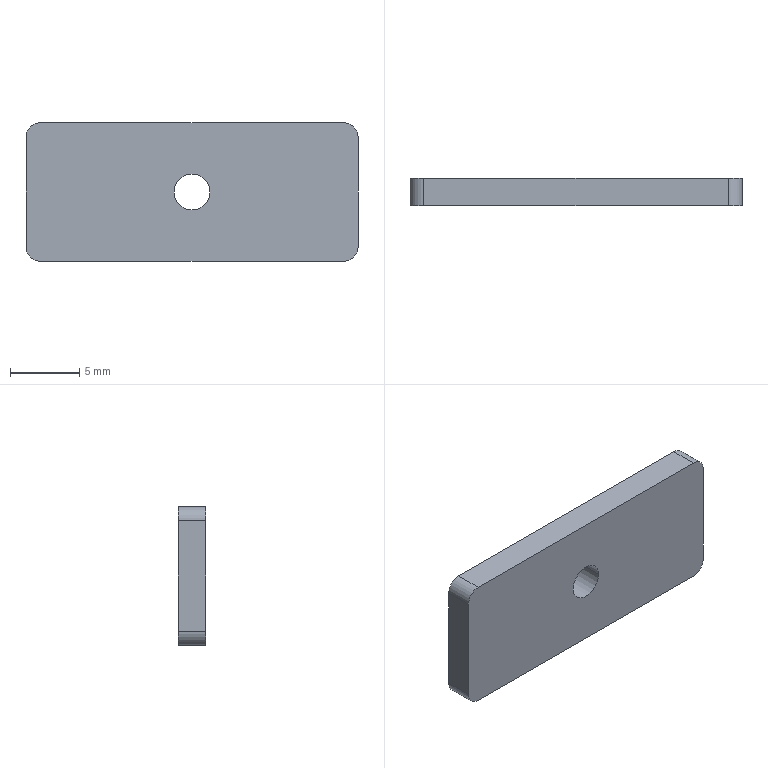Part | STEP file | LRS-150-12_X2_5F00517375-151336 | 1 solid | 12 faces | box 24 x 2 x 10 mm | volume 467.665 mm3 | cylinder 6 | plane 6 | commonest cylinder face diameters 2 x4 2.6 x2
STEP:
#1=CARTESIAN_POINT('',(0.,0.,0.));
#2=DIRECTION('',(0.,0.,1.));
#3=DIRECTION('',(1.,0.,0.));
#4=AXIS2_PLACEMENT_3D('',#1,#2,#3);
#5=CARTESIAN_POINT('',(-242.867,216.425,11.));
#6=VERTEX_POINT('',#5);
#7=CARTESIAN_POINT('',(-245.467,216.425,11.));
#8=VERTEX_POINT('',#7);
#9=CARTESIAN_POINT('',(-244.167,216.425,11.));
#10=DIRECTION('',(0.,-1.,0.));
#11=DIRECTION('',(1.,0.,0.));
#12=AXIS2_PLACEMENT_3D('',#9,#10,#11);
#13=CIRCLE('',#12,1.3);
#14=CARTESIAN_POINT('',(-244.167,214.225,11.));
#15=DIRECTION('',(0.,1.,0.));
#16=DIRECTION('',(1.,0.,0.));
#17=AXIS2_PLACEMENT_3D('',#14,#15,#16);
#18=CYLINDRICAL_SURFACE('',#17,1.3);
#19=CARTESIAN_POINT('',(6.283,2.2));
#20=DIRECTION('',(-1.,0.));
#21=VECTOR('',#20,1.);
#22=LINE('',#19,#21);
#23=(GEOMETRIC_REPRESENTATION_CONTEXT(2)PARAMETRIC_REPRESENTATION_CONTEXT()REPRESENTATION_CONTEXT('',''));
#24=DEFINITIONAL_REPRESENTATION('',(#22),#23);
#25=PCURVE('',#18,#24);
#26=CARTESIAN_POINT('',(-233.336,216.425,14.392));
#27=DIRECTION('',(0.,1.,0.));
#28=DIRECTION('',(1.,0.,0.));
#29=AXIS2_PLACEMENT_3D('',#26,#27,#28);
#30=PLANE('',#29);
#31=CARTESIAN_POINT('',(-9.53,3.392));
#32=CARTESIAN_POINT('',(-9.53,1.14));
#33=CARTESIAN_POINT('',(-11.48,2.266));
#34=CARTESIAN_POINT('',(-13.43,3.392));
#35=CARTESIAN_POINT('',(-11.48,4.517));
#36=CARTESIAN_POINT('',(-9.53,5.643));
#37=CARTESIAN_POINT('',(-9.53,3.392));
#38=(BOUNDED_CURVE()B_SPLINE_CURVE(2,(#31,#32,#33,#34,#35,#36,#37),.UNSPECIFIED.,.T.,.F.)B_SPLINE_CURVE_WITH_KNOTS((1,2,2,2,2,1),(-2.094,0.,2.094,4.189,6.283,8.378),.UNSPECIFIED.)CURVE()GEOMETRIC_REPRESENTATION_ITEM()RATIONAL_B_SPLINE_CURVE((1.,0.5,1.,0.5,1.,0.5,1.))REPRESENTATION_ITEM(''));
#39=(GEOMETRIC_REPRESENTATION_CONTEXT(2)PARAMETRIC_REPRESENTATION_CONTEXT()REPRESENTATION_CONTEXT('',''));
#40=DEFINITIONAL_REPRESENTATION('',(#38),#39);
#41=PCURVE('',#30,#40);
#42=SURFACE_CURVE('',#13,(#25,#41),.PCURVE_S1.);
#43=EDGE_CURVE('',#6,#8,#42,.T.);
#44=ORIENTED_EDGE('',*,*,#43,.T.);
#45=CARTESIAN_POINT('',(-245.467,214.425,11.));
#46=VERTEX_POINT('',#45);
#47=CARTESIAN_POINT('',(-245.467,216.425,11.));
#48=DIRECTION('',(0.,-1.,0.));
#49=VECTOR('',#48,1.);
#50=LINE('',#47,#49);
#51=CARTESIAN_POINT('',(3.142,2.2));
#52=DIRECTION('',(0.,-1.));
#53=VECTOR('',#52,1.);
#54=LINE('',#51,#53);
#55=(GEOMETRIC_REPRESENTATION_CONTEXT(2)PARAMETRIC_REPRESENTATION_CONTEXT()REPRESENTATION_CONTEXT('',''));
#56=DEFINITIONAL_REPRESENTATION('',(#54),#55);
#57=PCURVE('',#18,#56);
#58=CARTESIAN_POINT('',(-244.167,214.225,11.));
#59=DIRECTION('',(0.,1.,0.));
#60=DIRECTION('',(1.,0.,0.));
#61=AXIS2_PLACEMENT_3D('',#58,#59,#60);
#62=CYLINDRICAL_SURFACE('',#61,1.3);
#63=CARTESIAN_POINT('',(3.142,2.2));
#64=DIRECTION('',(0.,-1.));
#65=VECTOR('',#64,1.);
#66=LINE('',#63,#65);
#67=(GEOMETRIC_REPRESENTATION_CONTEXT(2)PARAMETRIC_REPRESENTATION_CONTEXT()REPRESENTATION_CONTEXT('',''));
#68=DEFINITIONAL_REPRESENTATION('',(#66),#67);
#69=PCURVE('',#62,#68);
#70=SURFACE_CURVE('',#50,(#57,#69),.PCURVE_S1.);
#71=EDGE_CURVE('',#8,#46,#70,.T.);
#72=ORIENTED_EDGE('',*,*,#71,.T.);
#73=CARTESIAN_POINT('',(-242.867,214.425,11.));
#74=VERTEX_POINT('',#73);
#75=CARTESIAN_POINT('',(-244.167,214.425,11.));
#76=DIRECTION('',(0.,1.,0.));
#77=DIRECTION('',(-1.,0.,0.));
#78=AXIS2_PLACEMENT_3D('',#75,#76,#77);
#79=CIRCLE('',#78,1.3);
#80=CARTESIAN_POINT('',(3.142,0.2));
#81=DIRECTION('',(1.,0.));
#82=VECTOR('',#81,1.);
#83=LINE('',#80,#82);
#84=(GEOMETRIC_REPRESENTATION_CONTEXT(2)PARAMETRIC_REPRESENTATION_CONTEXT()REPRESENTATION_CONTEXT('',''));
#85=DEFINITIONAL_REPRESENTATION('',(#83),#84);
#86=PCURVE('',#18,#85);
#87=CARTESIAN_POINT('',(-233.336,214.425,14.392));
#88=DIRECTION('',(0.,1.,0.));
#89=DIRECTION('',(1.,0.,0.));
#90=AXIS2_PLACEMENT_3D('',#87,#88,#89);
#91=PLANE('',#90);
#92=CARTESIAN_POINT('',(-10.83,3.392));
#93=DIRECTION('',(-1.,0.));
#94=AXIS2_PLACEMENT_2D('',#92,#93);
#95=CIRCLE('',#94,1.3);
#96=(GEOMETRIC_REPRESENTATION_CONTEXT(2)PARAMETRIC_REPRESENTATION_CONTEXT()REPRESENTATION_CONTEXT('',''));
#97=DEFINITIONAL_REPRESENTATION('',(#95),#96);
#98=PCURVE('',#91,#97);
#99=SURFACE_CURVE('',#79,(#86,#98),.PCURVE_S1.);
#100=EDGE_CURVE('',#46,#74,#99,.T.);
#101=ORIENTED_EDGE('',*,*,#100,.T.);
#102=CARTESIAN_POINT('',(-242.867,216.425,11.));
#103=DIRECTION('',(0.,-1.,0.));
#104=VECTOR('',#103,1.);
#105=LINE('',#102,#104);
#106=CARTESIAN_POINT('',(6.283,2.2));
#107=DIRECTION('',(0.,-1.));
#108=VECTOR('',#107,1.);
#109=LINE('',#106,#108);
#110=(GEOMETRIC_REPRESENTATION_CONTEXT(2)PARAMETRIC_REPRESENTATION_CONTEXT()REPRESENTATION_CONTEXT('',''));
#111=DEFINITIONAL_REPRESENTATION('',(#109),#110);
#112=PCURVE('',#18,#111);
#113=CARTESIAN_POINT('',(0.,2.2));
#114=DIRECTION('',(0.,-1.));
#115=VECTOR('',#114,1.);
#116=LINE('',#113,#115);
#117=(GEOMETRIC_REPRESENTATION_CONTEXT(2)PARAMETRIC_REPRESENTATION_CONTEXT()REPRESENTATION_CONTEXT('',''));
#118=DEFINITIONAL_REPRESENTATION('',(#116),#117);
#119=PCURVE('',#62,#118);
#120=SURFACE_CURVE('',#105,(#112,#119),.PCURVE_S1.);
#121=EDGE_CURVE('',#6,#74,#120,.T.);
#122=ORIENTED_EDGE('',*,*,#121,.F.);
#123=EDGE_LOOP('',(#44,#72,#101,#122));
#124=FACE_BOUND('',#123,.F.);
#125=ADVANCED_FACE('',(#124),#18,.F.);
#126=CARTESIAN_POINT('',(-256.167,216.425,15.));
#127=VERTEX_POINT('',#126);
#128=CARTESIAN_POINT('',(-255.167,216.425,16.));
#129=VERTEX_POINT('',#128);
#130=CARTESIAN_POINT('',(-255.167,216.425,15.));
#131=DIRECTION('',(0.,1.,0.));
#132=DIRECTION('',(-1.,0.,0.));
#133=AXIS2_PLACEMENT_3D('',#130,#131,#132);
#134=CIRCLE('',#133,1.);
#135=CARTESIAN_POINT('',(-21.83,-0.6085));
#136=DIRECTION('',(-1.,0.));
#137=AXIS2_PLACEMENT_2D('',#135,#136);
#138=CIRCLE('',#137,1.);
#139=(GEOMETRIC_REPRESENTATION_CONTEXT(2)PARAMETRIC_REPRESENTATION_CONTEXT()REPRESENTATION_CONTEXT('',''));
#140=DEFINITIONAL_REPRESENTATION('',(#138),#139);
#141=PCURVE('',#30,#140);
#142=CARTESIAN_POINT('',(-255.167,214.425,15.));
#143=DIRECTION('',(0.,1.,0.));
#144=DIRECTION('',(1.,0.,0.));
#145=AXIS2_PLACEMENT_3D('',#142,#143,#144);
#146=CYLINDRICAL_SURFACE('',#145,1.);
#147=CARTESIAN_POINT('',(3.142,2.));
#148=DIRECTION('',(1.,0.));
#149=VECTOR('',#148,1.);
#150=LINE('',#147,#149);
#151=(GEOMETRIC_REPRESENTATION_CONTEXT(2)PARAMETRIC_REPRESENTATION_CONTEXT()REPRESENTATION_CONTEXT('',''));
#152=DEFINITIONAL_REPRESENTATION('',(#150),#151);
#153=PCURVE('',#146,#152);
#154=SURFACE_CURVE('',#134,(#141,#153),.PCURVE_S1.);
#155=EDGE_CURVE('',#127,#129,#154,.T.);
#156=ORIENTED_EDGE('',*,*,#155,.F.);
#157=CARTESIAN_POINT('',(-256.167,216.425,7.));
#158=VERTEX_POINT('',#157);
#159=CARTESIAN_POINT('',(-256.167,216.425,7.));
#160=DIRECTION('',(0.,0.,1.));
#161=VECTOR('',#160,1.);
#162=LINE('',#159,#161);
#163=CARTESIAN_POINT('',(-22.83,7.392));
#164=DIRECTION('',(0.,-1.));
#165=VECTOR('',#164,1.);
#166=LINE('',#163,#165);
#167=(GEOMETRIC_REPRESENTATION_CONTEXT(2)PARAMETRIC_REPRESENTATION_CONTEXT()REPRESENTATION_CONTEXT('',''));
#168=DEFINITIONAL_REPRESENTATION('',(#166),#167);
#169=PCURVE('',#30,#168);
#170=CARTESIAN_POINT('',(-256.167,214.425,16.));
#171=DIRECTION('',(-1.,0.,0.));
#172=DIRECTION('',(0.,0.,1.));
#173=AXIS2_PLACEMENT_3D('',#170,#171,#172);
#174=PLANE('',#173);
#175=CARTESIAN_POINT('',(-9.,2.));
#176=DIRECTION('',(1.,0.));
#177=VECTOR('',#176,1.);
#178=LINE('',#175,#177);
#179=(GEOMETRIC_REPRESENTATION_CONTEXT(2)PARAMETRIC_REPRESENTATION_CONTEXT()REPRESENTATION_CONTEXT('',''));
#180=DEFINITIONAL_REPRESENTATION('',(#178),#179);
#181=PCURVE('',#174,#180);
#182=SURFACE_CURVE('',#162,(#169,#181),.PCURVE_S1.);
#183=EDGE_CURVE('',#158,#127,#182,.T.);
#184=ORIENTED_EDGE('',*,*,#183,.F.);
#185=CARTESIAN_POINT('',(-255.167,216.425,6.));
#186=VERTEX_POINT('',#185);
#187=CARTESIAN_POINT('',(-255.167,216.425,7.));
#188=DIRECTION('',(0.,1.,0.));
#189=DIRECTION('',(0.,0.,-1.));
#190=AXIS2_PLACEMENT_3D('',#187,#188,#189);
#191=CIRCLE('',#190,1.);
#192=CARTESIAN_POINT('',(-21.83,7.392));
#193=DIRECTION('',(0.,1.));
#194=AXIS2_PLACEMENT_2D('',#192,#193);
#195=CIRCLE('',#194,1.);
#196=(GEOMETRIC_REPRESENTATION_CONTEXT(2)PARAMETRIC_REPRESENTATION_CONTEXT()REPRESENTATION_CONTEXT('',''));
#197=DEFINITIONAL_REPRESENTATION('',(#195),#196);
#198=PCURVE('',#30,#197);
#199=CARTESIAN_POINT('',(-255.167,214.425,7.));
#200=DIRECTION('',(0.,1.,0.));
#201=DIRECTION('',(1.,0.,0.));
#202=AXIS2_PLACEMENT_3D('',#199,#200,#201);
#203=CYLINDRICAL_SURFACE('',#202,1.);
#204=CARTESIAN_POINT('',(1.571,2.));
#205=DIRECTION('',(1.,0.));
#206=VECTOR('',#205,1.);
#207=LINE('',#204,#206);
#208=(GEOMETRIC_REPRESENTATION_CONTEXT(2)PARAMETRIC_REPRESENTATION_CONTEXT()REPRESENTATION_CONTEXT('',''));
#209=DEFINITIONAL_REPRESENTATION('',(#207),#208);
#210=PCURVE('',#203,#209);
#211=SURFACE_CURVE('',#191,(#198,#210),.PCURVE_S1.);
#212=EDGE_CURVE('',#186,#158,#211,.T.);
#213=ORIENTED_EDGE('',*,*,#212,.F.);
#214=CARTESIAN_POINT('',(-233.167,216.425,6.));
#215=VERTEX_POINT('',#214);
#216=CARTESIAN_POINT('',(-255.167,216.425,6.));
#217=DIRECTION('',(1.,0.,0.));
#218=VECTOR('',#217,1.);
#219=LINE('',#216,#218);
#220=CARTESIAN_POINT('',(-21.83,8.392));
#221=DIRECTION('',(1.,0.));
#222=VECTOR('',#221,1.);
#223=LINE('',#220,#222);
#224=(GEOMETRIC_REPRESENTATION_CONTEXT(2)PARAMETRIC_REPRESENTATION_CONTEXT()REPRESENTATION_CONTEXT('',''));
#225=DEFINITIONAL_REPRESENTATION('',(#223),#224);
#226=PCURVE('',#30,#225);
#227=CARTESIAN_POINT('',(-261.667,214.425,6.));
#228=DIRECTION('',(0.,0.,-1.));
#229=DIRECTION('',(-1.,0.,0.));
#230=AXIS2_PLACEMENT_3D('',#227,#228,#229);
#231=PLANE('',#230);
#232=CARTESIAN_POINT('',(-6.5,2.));
#233=DIRECTION('',(-1.,0.));
#234=VECTOR('',#233,1.);
#235=LINE('',#232,#234);
#236=(GEOMETRIC_REPRESENTATION_CONTEXT(2)PARAMETRIC_REPRESENTATION_CONTEXT()REPRESENTATION_CONTEXT('',''));
#237=DEFINITIONAL_REPRESENTATION('',(#235),#236);
#238=PCURVE('',#231,#237);
#239=SURFACE_CURVE('',#219,(#226,#238),.PCURVE_S1.);
#240=EDGE_CURVE('',#186,#215,#239,.T.);
#241=ORIENTED_EDGE('',*,*,#240,.T.);
#242=CARTESIAN_POINT('',(-232.167,216.425,7.));
#243=VERTEX_POINT('',#242);
#244=CARTESIAN_POINT('',(-233.167,216.425,7.));
#245=DIRECTION('',(0.,1.,0.));
#246=DIRECTION('',(1.,0.,0.));
#247=AXIS2_PLACEMENT_3D('',#244,#245,#246);
#248=CIRCLE('',#247,1.);
#249=CARTESIAN_POINT('',(0.1696,7.392));
#250=DIRECTION('',(1.,0.));
#251=AXIS2_PLACEMENT_2D('',#249,#250);
#252=CIRCLE('',#251,1.);
#253=(GEOMETRIC_REPRESENTATION_CONTEXT(2)PARAMETRIC_REPRESENTATION_CONTEXT()REPRESENTATION_CONTEXT('',''));
#254=DEFINITIONAL_REPRESENTATION('',(#252),#253);
#255=PCURVE('',#30,#254);
#256=CARTESIAN_POINT('',(-233.167,214.425,7.));
#257=DIRECTION('',(0.,1.,0.));
#258=DIRECTION('',(1.,0.,0.));
#259=AXIS2_PLACEMENT_3D('',#256,#257,#258);
#260=CYLINDRICAL_SURFACE('',#259,1.);
#261=CARTESIAN_POINT('',(0.,2.));
#262=DIRECTION('',(1.,0.));
#263=VECTOR('',#262,1.);
#264=LINE('',#261,#263);
#265=(GEOMETRIC_REPRESENTATION_CONTEXT(2)PARAMETRIC_REPRESENTATION_CONTEXT()REPRESENTATION_CONTEXT('',''));
#266=DEFINITIONAL_REPRESENTATION('',(#264),#265);
#267=PCURVE('',#260,#266);
#268=SURFACE_CURVE('',#248,(#255,#267),.PCURVE_S1.);
#269=EDGE_CURVE('',#243,#215,#268,.T.);
#270=ORIENTED_EDGE('',*,*,#269,.F.);
#271=CARTESIAN_POINT('',(-232.167,216.425,15.));
#272=VERTEX_POINT('',#271);
#273=CARTESIAN_POINT('',(-232.167,216.425,15.));
#274=DIRECTION('',(0.,0.,-1.));
#275=VECTOR('',#274,1.);
#276=LINE('',#273,#275);
#277=CARTESIAN_POINT('',(1.17,-0.6085));
#278=DIRECTION('',(0.,1.));
#279=VECTOR('',#278,1.);
#280=LINE('',#277,#279);
#281=(GEOMETRIC_REPRESENTATION_CONTEXT(2)PARAMETRIC_REPRESENTATION_CONTEXT()REPRESENTATION_CONTEXT('',''));
#282=DEFINITIONAL_REPRESENTATION('',(#280),#281);
#283=PCURVE('',#30,#282);
#284=CARTESIAN_POINT('',(-232.167,214.425,6.));
#285=DIRECTION('',(1.,0.,0.));
#286=DIRECTION('',(0.,0.,-1.));
#287=AXIS2_PLACEMENT_3D('',#284,#285,#286);
#288=PLANE('',#287);
#289=CARTESIAN_POINT('',(-9.,2.));
#290=DIRECTION('',(1.,0.));
#291=VECTOR('',#290,1.);
#292=LINE('',#289,#291);
#293=(GEOMETRIC_REPRESENTATION_CONTEXT(2)PARAMETRIC_REPRESENTATION_CONTEXT()REPRESENTATION_CONTEXT('',''));
#294=DEFINITIONAL_REPRESENTATION('',(#292),#293);
#295=PCURVE('',#288,#294);
#296=SURFACE_CURVE('',#276,(#283,#295),.PCURVE_S1.);
#297=EDGE_CURVE('',#272,#243,#296,.T.);
#298=ORIENTED_EDGE('',*,*,#297,.F.);
#299=CARTESIAN_POINT('',(-233.167,216.425,16.));
#300=VERTEX_POINT('',#299);
#301=CARTESIAN_POINT('',(-233.167,216.425,15.));
#302=DIRECTION('',(0.,1.,0.));
#303=DIRECTION('',(0.,0.,1.));
#304=AXIS2_PLACEMENT_3D('',#301,#302,#303);
#305=CIRCLE('',#304,1.);
#306=CARTESIAN_POINT('',(0.1696,-0.6085));
#307=DIRECTION('',(0.,-1.));
#308=AXIS2_PLACEMENT_2D('',#306,#307);
#309=CIRCLE('',#308,1.);
#310=(GEOMETRIC_REPRESENTATION_CONTEXT(2)PARAMETRIC_REPRESENTATION_CONTEXT()REPRESENTATION_CONTEXT('',''));
#311=DEFINITIONAL_REPRESENTATION('',(#309),#310);
#312=PCURVE('',#30,#311);
#313=CARTESIAN_POINT('',(-233.167,214.425,15.));
#314=DIRECTION('',(0.,1.,0.));
#315=DIRECTION('',(1.,0.,0.));
#316=AXIS2_PLACEMENT_3D('',#313,#314,#315);
#317=CYLINDRICAL_SURFACE('',#316,1.);
#318=CARTESIAN_POINT('',(4.712,2.));
#319=DIRECTION('',(1.,0.));
#320=VECTOR('',#319,1.);
#321=LINE('',#318,#320);
#322=(GEOMETRIC_REPRESENTATION_CONTEXT(2)PARAMETRIC_REPRESENTATION_CONTEXT()REPRESENTATION_CONTEXT('',''));
#323=DEFINITIONAL_REPRESENTATION('',(#321),#322);
#324=PCURVE('',#317,#323);
#325=SURFACE_CURVE('',#305,(#312,#324),.PCURVE_S1.);
#326=EDGE_CURVE('',#300,#272,#325,.T.);
#327=ORIENTED_EDGE('',*,*,#326,.F.);
#328=CARTESIAN_POINT('',(-233.167,216.425,16.));
#329=DIRECTION('',(-1.,0.,0.));
#330=VECTOR('',#329,1.);
#331=LINE('',#328,#330);
#332=CARTESIAN_POINT('',(0.1696,-1.608));
#333=DIRECTION('',(-1.,0.));
#334=VECTOR('',#333,1.);
#335=LINE('',#332,#334);
#336=(GEOMETRIC_REPRESENTATION_CONTEXT(2)PARAMETRIC_REPRESENTATION_CONTEXT()REPRESENTATION_CONTEXT('',''));
#337=DEFINITIONAL_REPRESENTATION('',(#335),#336);
#338=PCURVE('',#30,#337);
#339=CARTESIAN_POINT('',(-226.667,214.425,16.));
#340=DIRECTION('',(0.,0.,1.));
#341=DIRECTION('',(1.,0.,0.));
#342=AXIS2_PLACEMENT_3D('',#339,#340,#341);
#343=PLANE('',#342);
#344=CARTESIAN_POINT('',(-6.5,2.));
#345=DIRECTION('',(-1.,0.));
#346=VECTOR('',#345,1.);
#347=LINE('',#344,#346);
#348=(GEOMETRIC_REPRESENTATION_CONTEXT(2)PARAMETRIC_REPRESENTATION_CONTEXT()REPRESENTATION_CONTEXT('',''));
#349=DEFINITIONAL_REPRESENTATION('',(#347),#348);
#350=PCURVE('',#343,#349);
#351=SURFACE_CURVE('',#331,(#338,#350),.PCURVE_S1.);
#352=EDGE_CURVE('',#300,#129,#351,.T.);
#353=ORIENTED_EDGE('',*,*,#352,.T.);
#354=EDGE_LOOP('',(#156,#184,#213,#241,#270,#298,#327,#353));
#355=FACE_BOUND('',#354,.F.);
#356=ORIENTED_EDGE('',*,*,#43,.F.);
#357=CARTESIAN_POINT('',(-244.167,216.425,11.));
#358=DIRECTION('',(0.,-1.,0.));
#359=DIRECTION('',(-1.,0.,0.));
#360=AXIS2_PLACEMENT_3D('',#357,#358,#359);
#361=CIRCLE('',#360,1.3);
#362=CARTESIAN_POINT('',(-12.13,3.392));
#363=CARTESIAN_POINT('',(-12.13,5.643));
#364=CARTESIAN_POINT('',(-10.18,4.517));
#365=CARTESIAN_POINT('',(-8.23,3.392));
#366=CARTESIAN_POINT('',(-10.18,2.266));
#367=CARTESIAN_POINT('',(-12.13,1.14));
#368=CARTESIAN_POINT('',(-12.13,3.392));
#369=(BOUNDED_CURVE()B_SPLINE_CURVE(2,(#362,#363,#364,#365,#366,#367,#368),.UNSPECIFIED.,.T.,.F.)B_SPLINE_CURVE_WITH_KNOTS((1,2,2,2,2,1),(-2.094,0.,2.094,4.189,6.283,8.378),.UNSPECIFIED.)CURVE()GEOMETRIC_REPRESENTATION_ITEM()RATIONAL_B_SPLINE_CURVE((1.,0.5,1.,0.5,1.,0.5,1.))REPRESENTATION_ITEM(''));
#370=(GEOMETRIC_REPRESENTATION_CONTEXT(2)PARAMETRIC_REPRESENTATION_CONTEXT()REPRESENTATION_CONTEXT('',''));
#371=DEFINITIONAL_REPRESENTATION('',(#369),#370);
#372=PCURVE('',#30,#371);
#373=CARTESIAN_POINT('',(3.142,2.2));
#374=DIRECTION('',(-1.,0.));
#375=VECTOR('',#374,1.);
#376=LINE('',#373,#375);
#377=(GEOMETRIC_REPRESENTATION_CONTEXT(2)PARAMETRIC_REPRESENTATION_CONTEXT()REPRESENTATION_CONTEXT('',''));
#378=DEFINITIONAL_REPRESENTATION('',(#376),#377);
#379=PCURVE('',#62,#378);
#380=SURFACE_CURVE('',#361,(#372,#379),.PCURVE_S1.);
#381=EDGE_CURVE('',#8,#6,#380,.T.);
#382=ORIENTED_EDGE('',*,*,#381,.F.);
#383=EDGE_LOOP('',(#356,#382));
#384=FACE_BOUND('',#383,.F.);
#385=ADVANCED_FACE('',(#355,#384),#30,.T.);
#386=ORIENTED_EDGE('',*,*,#121,.T.);
#387=CARTESIAN_POINT('',(-244.167,214.425,11.));
#388=DIRECTION('',(0.,1.,0.));
#389=DIRECTION('',(1.,0.,0.));
#390=AXIS2_PLACEMENT_3D('',#387,#388,#389);
#391=CIRCLE('',#390,1.3);
#392=CARTESIAN_POINT('',(0.,0.2));
#393=DIRECTION('',(1.,0.));
#394=VECTOR('',#393,1.);
#395=LINE('',#392,#394);
#396=(GEOMETRIC_REPRESENTATION_CONTEXT(2)PARAMETRIC_REPRESENTATION_CONTEXT()REPRESENTATION_CONTEXT('',''));
#397=DEFINITIONAL_REPRESENTATION('',(#395),#396);
#398=PCURVE('',#62,#397);
#399=CARTESIAN_POINT('',(-10.83,3.392));
#400=DIRECTION('',(1.,0.));
#401=AXIS2_PLACEMENT_2D('',#399,#400);
#402=CIRCLE('',#401,1.3);
#403=(GEOMETRIC_REPRESENTATION_CONTEXT(2)PARAMETRIC_REPRESENTATION_CONTEXT()REPRESENTATION_CONTEXT('',''));
#404=DEFINITIONAL_REPRESENTATION('',(#402),#403);
#405=PCURVE('',#91,#404);
#406=SURFACE_CURVE('',#391,(#398,#405),.PCURVE_S1.);
#407=EDGE_CURVE('',#74,#46,#406,.T.);
#408=ORIENTED_EDGE('',*,*,#407,.T.);
#409=ORIENTED_EDGE('',*,*,#71,.F.);
#410=ORIENTED_EDGE('',*,*,#381,.T.);
#411=EDGE_LOOP('',(#386,#408,#409,#410));
#412=FACE_BOUND('',#411,.F.);
#413=ADVANCED_FACE('',(#412),#62,.F.);
#414=CARTESIAN_POINT('',(-233.167,214.425,6.));
#415=VERTEX_POINT('',#414);
#416=CARTESIAN_POINT('',(-232.167,214.425,7.));
#417=VERTEX_POINT('',#416);
#418=CARTESIAN_POINT('',(-233.167,214.425,7.));
#419=DIRECTION('',(0.,-1.,0.));
#420=DIRECTION('',(0.,0.,-1.));
#421=AXIS2_PLACEMENT_3D('',#418,#419,#420);
#422=CIRCLE('',#421,1.);
#423=CARTESIAN_POINT('',(0.1696,8.392));
#424=CARTESIAN_POINT('',(1.902,8.392));
#425=CARTESIAN_POINT('',(1.036,6.892));
#426=CARTESIAN_POINT('',(0.1696,5.392));
#427=CARTESIAN_POINT('',(-0.6964,6.892));
#428=CARTESIAN_POINT('',(-1.562,8.392));
#429=CARTESIAN_POINT('',(0.1696,8.392));
#430=(BOUNDED_CURVE()B_SPLINE_CURVE(2,(#423,#424,#425,#426,#427,#428,#429),.UNSPECIFIED.,.T.,.F.)B_SPLINE_CURVE_WITH_KNOTS((1,2,2,2,2,1),(-2.094,0.,2.094,4.189,6.283,8.378),.UNSPECIFIED.)CURVE()GEOMETRIC_REPRESENTATION_ITEM()RATIONAL_B_SPLINE_CURVE((1.,0.5,1.,0.5,1.,0.5,1.))REPRESENTATION_ITEM(''));
#431=(GEOMETRIC_REPRESENTATION_CONTEXT(2)PARAMETRIC_REPRESENTATION_CONTEXT()REPRESENTATION_CONTEXT('',''));
#432=DEFINITIONAL_REPRESENTATION('',(#430),#431);
#433=PCURVE('',#91,#432);
#434=CARTESIAN_POINT('',(1.571,0.));
#435=DIRECTION('',(-1.,0.));
#436=VECTOR('',#435,1.);
#437=LINE('',#434,#436);
#438=(GEOMETRIC_REPRESENTATION_CONTEXT(2)PARAMETRIC_REPRESENTATION_CONTEXT()REPRESENTATION_CONTEXT('',''));
#439=DEFINITIONAL_REPRESENTATION('',(#437),#438);
#440=PCURVE('',#260,#439);
#441=SURFACE_CURVE('',#422,(#433,#440),.PCURVE_S1.);
#442=EDGE_CURVE('',#415,#417,#441,.T.);
#443=ORIENTED_EDGE('',*,*,#442,.F.);
#444=CARTESIAN_POINT('',(-255.167,214.425,6.));
#445=VERTEX_POINT('',#444);
#446=CARTESIAN_POINT('',(-255.167,214.425,6.));
#447=DIRECTION('',(1.,0.,0.));
#448=VECTOR('',#447,1.);
#449=LINE('',#446,#448);
#450=CARTESIAN_POINT('',(-21.83,8.392));
#451=DIRECTION('',(1.,0.));
#452=VECTOR('',#451,1.);
#453=LINE('',#450,#452);
#454=(GEOMETRIC_REPRESENTATION_CONTEXT(2)PARAMETRIC_REPRESENTATION_CONTEXT()REPRESENTATION_CONTEXT('',''));
#455=DEFINITIONAL_REPRESENTATION('',(#453),#454);
#456=PCURVE('',#91,#455);
#457=CARTESIAN_POINT('',(-6.5,0.));
#458=DIRECTION('',(-1.,0.));
#459=VECTOR('',#458,1.);
#460=LINE('',#457,#459);
#461=(GEOMETRIC_REPRESENTATION_CONTEXT(2)PARAMETRIC_REPRESENTATION_CONTEXT()REPRESENTATION_CONTEXT('',''));
#462=DEFINITIONAL_REPRESENTATION('',(#460),#461);
#463=PCURVE('',#231,#462);
#464=SURFACE_CURVE('',#449,(#456,#463),.PCURVE_S1.);
#465=EDGE_CURVE('',#445,#415,#464,.T.);
#466=ORIENTED_EDGE('',*,*,#465,.F.);
#467=CARTESIAN_POINT('',(-256.167,214.425,7.));
#468=VERTEX_POINT('',#467);
#469=CARTESIAN_POINT('',(-255.167,214.425,7.));
#470=DIRECTION('',(0.,-1.,0.));
#471=DIRECTION('',(-1.,0.,0.));
#472=AXIS2_PLACEMENT_3D('',#469,#470,#471);
#473=CIRCLE('',#472,1.);
#474=CARTESIAN_POINT('',(-22.83,7.392));
#475=CARTESIAN_POINT('',(-22.83,9.124));
#476=CARTESIAN_POINT('',(-21.33,8.258));
#477=CARTESIAN_POINT('',(-19.83,7.392));
#478=CARTESIAN_POINT('',(-21.33,6.526));
#479=CARTESIAN_POINT('',(-22.83,5.659));
#480=CARTESIAN_POINT('',(-22.83,7.392));
#481=(BOUNDED_CURVE()B_SPLINE_CURVE(2,(#474,#475,#476,#477,#478,#479,#480),.UNSPECIFIED.,.T.,.F.)B_SPLINE_CURVE_WITH_KNOTS((1,2,2,2,2,1),(-2.094,0.,2.094,4.189,6.283,8.378),.UNSPECIFIED.)CURVE()GEOMETRIC_REPRESENTATION_ITEM()RATIONAL_B_SPLINE_CURVE((1.,0.5,1.,0.5,1.,0.5,1.))REPRESENTATION_ITEM(''));
#482=(GEOMETRIC_REPRESENTATION_CONTEXT(2)PARAMETRIC_REPRESENTATION_CONTEXT()REPRESENTATION_CONTEXT('',''));
#483=DEFINITIONAL_REPRESENTATION('',(#481),#482);
#484=PCURVE('',#91,#483);
#485=CARTESIAN_POINT('',(3.142,0.));
#486=DIRECTION('',(-1.,0.));
#487=VECTOR('',#486,1.);
#488=LINE('',#485,#487);
#489=(GEOMETRIC_REPRESENTATION_CONTEXT(2)PARAMETRIC_REPRESENTATION_CONTEXT()REPRESENTATION_CONTEXT('',''));
#490=DEFINITIONAL_REPRESENTATION('',(#488),#489);
#491=PCURVE('',#203,#490);
#492=SURFACE_CURVE('',#473,(#484,#491),.PCURVE_S1.);
#493=EDGE_CURVE('',#468,#445,#492,.T.);
#494=ORIENTED_EDGE('',*,*,#493,.F.);
#495=CARTESIAN_POINT('',(-256.167,214.425,15.));
#496=VERTEX_POINT('',#495);
#497=CARTESIAN_POINT('',(-256.167,214.425,7.));
#498=DIRECTION('',(0.,0.,1.));
#499=VECTOR('',#498,1.);
#500=LINE('',#497,#499);
#501=CARTESIAN_POINT('',(-22.83,7.392));
#502=DIRECTION('',(0.,-1.));
#503=VECTOR('',#502,1.);
#504=LINE('',#501,#503);
#505=(GEOMETRIC_REPRESENTATION_CONTEXT(2)PARAMETRIC_REPRESENTATION_CONTEXT()REPRESENTATION_CONTEXT('',''));
#506=DEFINITIONAL_REPRESENTATION('',(#504),#505);
#507=PCURVE('',#91,#506);
#508=CARTESIAN_POINT('',(-9.,0.));
#509=DIRECTION('',(1.,0.));
#510=VECTOR('',#509,1.);
#511=LINE('',#508,#510);
#512=(GEOMETRIC_REPRESENTATION_CONTEXT(2)PARAMETRIC_REPRESENTATION_CONTEXT()REPRESENTATION_CONTEXT('',''));
#513=DEFINITIONAL_REPRESENTATION('',(#511),#512);
#514=PCURVE('',#174,#513);
#515=SURFACE_CURVE('',#500,(#507,#514),.PCURVE_S1.);
#516=EDGE_CURVE('',#468,#496,#515,.T.);
#517=ORIENTED_EDGE('',*,*,#516,.T.);
#518=CARTESIAN_POINT('',(-255.167,214.425,16.));
#519=VERTEX_POINT('',#518);
#520=CARTESIAN_POINT('',(-255.167,214.425,15.));
#521=DIRECTION('',(0.,-1.,0.));
#522=DIRECTION('',(0.,0.,1.));
#523=AXIS2_PLACEMENT_3D('',#520,#521,#522);
#524=CIRCLE('',#523,1.);
#525=CARTESIAN_POINT('',(-21.83,-1.608));
#526=CARTESIAN_POINT('',(-23.562,-1.608));
#527=CARTESIAN_POINT('',(-22.696,-0.1085));
#528=CARTESIAN_POINT('',(-21.83,1.392));
#529=CARTESIAN_POINT('',(-20.964,-0.1085));
#530=CARTESIAN_POINT('',(-20.098,-1.608));
#531=CARTESIAN_POINT('',(-21.83,-1.608));
#532=(BOUNDED_CURVE()B_SPLINE_CURVE(2,(#525,#526,#527,#528,#529,#530,#531),.UNSPECIFIED.,.T.,.F.)B_SPLINE_CURVE_WITH_KNOTS((1,2,2,2,2,1),(-2.094,0.,2.094,4.189,6.283,8.378),.UNSPECIFIED.)CURVE()GEOMETRIC_REPRESENTATION_ITEM()RATIONAL_B_SPLINE_CURVE((1.,0.5,1.,0.5,1.,0.5,1.))REPRESENTATION_ITEM(''));
#533=(GEOMETRIC_REPRESENTATION_CONTEXT(2)PARAMETRIC_REPRESENTATION_CONTEXT()REPRESENTATION_CONTEXT('',''));
#534=DEFINITIONAL_REPRESENTATION('',(#532),#533);
#535=PCURVE('',#91,#534);
#536=CARTESIAN_POINT('',(4.712,0.));
#537=DIRECTION('',(-1.,0.));
#538=VECTOR('',#537,1.);
#539=LINE('',#536,#538);
#540=(GEOMETRIC_REPRESENTATION_CONTEXT(2)PARAMETRIC_REPRESENTATION_CONTEXT()REPRESENTATION_CONTEXT('',''));
#541=DEFINITIONAL_REPRESENTATION('',(#539),#540);
#542=PCURVE('',#146,#541);
#543=SURFACE_CURVE('',#524,(#535,#542),.PCURVE_S1.);
#544=EDGE_CURVE('',#519,#496,#543,.T.);
#545=ORIENTED_EDGE('',*,*,#544,.F.);
#546=CARTESIAN_POINT('',(-233.167,214.425,16.));
#547=VERTEX_POINT('',#546);
#548=CARTESIAN_POINT('',(-233.167,214.425,16.));
#549=DIRECTION('',(-1.,0.,0.));
#550=VECTOR('',#549,1.);
#551=LINE('',#548,#550);
#552=CARTESIAN_POINT('',(0.1696,-1.608));
#553=DIRECTION('',(-1.,0.));
#554=VECTOR('',#553,1.);
#555=LINE('',#552,#554);
#556=(GEOMETRIC_REPRESENTATION_CONTEXT(2)PARAMETRIC_REPRESENTATION_CONTEXT()REPRESENTATION_CONTEXT('',''));
#557=DEFINITIONAL_REPRESENTATION('',(#555),#556);
#558=PCURVE('',#91,#557);
#559=CARTESIAN_POINT('',(-6.5,0.));
#560=DIRECTION('',(-1.,0.));
#561=VECTOR('',#560,1.);
#562=LINE('',#559,#561);
#563=(GEOMETRIC_REPRESENTATION_CONTEXT(2)PARAMETRIC_REPRESENTATION_CONTEXT()REPRESENTATION_CONTEXT('',''));
#564=DEFINITIONAL_REPRESENTATION('',(#562),#563);
#565=PCURVE('',#343,#564);
#566=SURFACE_CURVE('',#551,(#558,#565),.PCURVE_S1.);
#567=EDGE_CURVE('',#547,#519,#566,.T.);
#568=ORIENTED_EDGE('',*,*,#567,.F.);
#569=CARTESIAN_POINT('',(-232.167,214.425,15.));
#570=VERTEX_POINT('',#569);
#571=CARTESIAN_POINT('',(-233.167,214.425,15.));
#572=DIRECTION('',(0.,-1.,0.));
#573=DIRECTION('',(1.,0.,0.));
#574=AXIS2_PLACEMENT_3D('',#571,#572,#573);
#575=CIRCLE('',#574,1.);
#576=CARTESIAN_POINT('',(1.17,-0.6085));
#577=CARTESIAN_POINT('',(1.17,-2.341));
#578=CARTESIAN_POINT('',(-0.3304,-1.474));
#579=CARTESIAN_POINT('',(-1.83,-0.6085));
#580=CARTESIAN_POINT('',(-0.3304,0.2576));
#581=CARTESIAN_POINT('',(1.17,1.124));
#582=CARTESIAN_POINT('',(1.17,-0.6085));
#583=(BOUNDED_CURVE()B_SPLINE_CURVE(2,(#576,#577,#578,#579,#580,#581,#582),.UNSPECIFIED.,.T.,.F.)B_SPLINE_CURVE_WITH_KNOTS((1,2,2,2,2,1),(-2.094,0.,2.094,4.189,6.283,8.378),.UNSPECIFIED.)CURVE()GEOMETRIC_REPRESENTATION_ITEM()RATIONAL_B_SPLINE_CURVE((1.,0.5,1.,0.5,1.,0.5,1.))REPRESENTATION_ITEM(''));
#584=(GEOMETRIC_REPRESENTATION_CONTEXT(2)PARAMETRIC_REPRESENTATION_CONTEXT()REPRESENTATION_CONTEXT('',''));
#585=DEFINITIONAL_REPRESENTATION('',(#583),#584);
#586=PCURVE('',#91,#585);
#587=CARTESIAN_POINT('',(6.283,0.));
#588=DIRECTION('',(-1.,0.));
#589=VECTOR('',#588,1.);
#590=LINE('',#587,#589);
#591=(GEOMETRIC_REPRESENTATION_CONTEXT(2)PARAMETRIC_REPRESENTATION_CONTEXT()REPRESENTATION_CONTEXT('',''));
#592=DEFINITIONAL_REPRESENTATION('',(#590),#591);
#593=PCURVE('',#317,#592);
#594=SURFACE_CURVE('',#575,(#586,#593),.PCURVE_S1.);
#595=EDGE_CURVE('',#570,#547,#594,.T.);
#596=ORIENTED_EDGE('',*,*,#595,.F.);
#597=CARTESIAN_POINT('',(-232.167,214.425,15.));
#598=DIRECTION('',(0.,0.,-1.));
#599=VECTOR('',#598,1.);
#600=LINE('',#597,#599);
#601=CARTESIAN_POINT('',(1.17,-0.6085));
#602=DIRECTION('',(0.,1.));
#603=VECTOR('',#602,1.);
#604=LINE('',#601,#603);
#605=(GEOMETRIC_REPRESENTATION_CONTEXT(2)PARAMETRIC_REPRESENTATION_CONTEXT()REPRESENTATION_CONTEXT('',''));
#606=DEFINITIONAL_REPRESENTATION('',(#604),#605);
#607=PCURVE('',#91,#606);
#608=CARTESIAN_POINT('',(-9.,0.));
#609=DIRECTION('',(1.,0.));
#610=VECTOR('',#609,1.);
#611=LINE('',#608,#610);
#612=(GEOMETRIC_REPRESENTATION_CONTEXT(2)PARAMETRIC_REPRESENTATION_CONTEXT()REPRESENTATION_CONTEXT('',''));
#613=DEFINITIONAL_REPRESENTATION('',(#611),#612);
#614=PCURVE('',#288,#613);
#615=SURFACE_CURVE('',#600,(#607,#614),.PCURVE_S1.);
#616=EDGE_CURVE('',#570,#417,#615,.T.);
#617=ORIENTED_EDGE('',*,*,#616,.T.);
#618=EDGE_LOOP('',(#443,#466,#494,#517,#545,#568,#596,#617));
#619=FACE_BOUND('',#618,.F.);
#620=ORIENTED_EDGE('',*,*,#100,.F.);
#621=ORIENTED_EDGE('',*,*,#407,.F.);
#622=EDGE_LOOP('',(#620,#621));
#623=FACE_BOUND('',#622,.F.);
#624=ADVANCED_FACE('',(#619,#623),#91,.F.);
#625=CARTESIAN_POINT('',(-232.167,216.425,7.));
#626=DIRECTION('',(0.,-1.,0.));
#627=VECTOR('',#626,1.);
#628=LINE('',#625,#627);
#629=CARTESIAN_POINT('',(0.,2.));
#630=DIRECTION('',(0.,-1.));
#631=VECTOR('',#630,1.);
#632=LINE('',#629,#631);
#633=(GEOMETRIC_REPRESENTATION_CONTEXT(2)PARAMETRIC_REPRESENTATION_CONTEXT()REPRESENTATION_CONTEXT('',''));
#634=DEFINITIONAL_REPRESENTATION('',(#632),#633);
#635=PCURVE('',#260,#634);
#636=CARTESIAN_POINT('',(-1.,2.));
#637=DIRECTION('',(0.,-1.));
#638=VECTOR('',#637,1.);
#639=LINE('',#636,#638);
#640=(GEOMETRIC_REPRESENTATION_CONTEXT(2)PARAMETRIC_REPRESENTATION_CONTEXT()REPRESENTATION_CONTEXT('',''));
#641=DEFINITIONAL_REPRESENTATION('',(#639),#640);
#642=PCURVE('',#288,#641);
#643=SURFACE_CURVE('',#628,(#635,#642),.PCURVE_S1.);
#644=EDGE_CURVE('',#243,#417,#643,.T.);
#645=ORIENTED_EDGE('',*,*,#644,.T.);
#646=ORIENTED_EDGE('',*,*,#442,.F.);
#647=CARTESIAN_POINT('',(-233.167,214.425,6.));
#648=DIRECTION('',(0.,1.,0.));
#649=VECTOR('',#648,1.);
#650=LINE('',#647,#649);
#651=CARTESIAN_POINT('',(1.571,0.));
#652=DIRECTION('',(0.,1.));
#653=VECTOR('',#652,1.);
#654=LINE('',#651,#653);
#655=(GEOMETRIC_REPRESENTATION_CONTEXT(2)PARAMETRIC_REPRESENTATION_CONTEXT()REPRESENTATION_CONTEXT('',''));
#656=DEFINITIONAL_REPRESENTATION('',(#654),#655);
#657=PCURVE('',#260,#656);
#658=CARTESIAN_POINT('',(-28.5,0.));
#659=DIRECTION('',(0.,1.));
#660=VECTOR('',#659,1.);
#661=LINE('',#658,#660);
#662=(GEOMETRIC_REPRESENTATION_CONTEXT(2)PARAMETRIC_REPRESENTATION_CONTEXT()REPRESENTATION_CONTEXT('',''));
#663=DEFINITIONAL_REPRESENTATION('',(#661),#662);
#664=PCURVE('',#231,#663);
#665=SURFACE_CURVE('',#650,(#657,#664),.PCURVE_S1.);
#666=EDGE_CURVE('',#415,#215,#665,.T.);
#667=ORIENTED_EDGE('',*,*,#666,.T.);
#668=ORIENTED_EDGE('',*,*,#269,.F.);
#669=EDGE_LOOP('',(#645,#646,#667,#668));
#670=FACE_BOUND('',#669,.T.);
#671=ADVANCED_FACE('',(#670),#260,.T.);
#672=ORIENTED_EDGE('',*,*,#465,.T.);
#673=ORIENTED_EDGE('',*,*,#666,.T.);
#674=ORIENTED_EDGE('',*,*,#240,.F.);
#675=CARTESIAN_POINT('',(-255.167,216.425,6.));
#676=DIRECTION('',(0.,-1.,0.));
#677=VECTOR('',#676,1.);
#678=LINE('',#675,#677);
#679=CARTESIAN_POINT('',(-6.5,2.));
#680=DIRECTION('',(0.,-1.));
#681=VECTOR('',#680,1.);
#682=LINE('',#679,#681);
#683=(GEOMETRIC_REPRESENTATION_CONTEXT(2)PARAMETRIC_REPRESENTATION_CONTEXT()REPRESENTATION_CONTEXT('',''));
#684=DEFINITIONAL_REPRESENTATION('',(#682),#683);
#685=PCURVE('',#231,#684);
#686=CARTESIAN_POINT('',(1.571,2.));
#687=DIRECTION('',(0.,-1.));
#688=VECTOR('',#687,1.);
#689=LINE('',#686,#688);
#690=(GEOMETRIC_REPRESENTATION_CONTEXT(2)PARAMETRIC_REPRESENTATION_CONTEXT()REPRESENTATION_CONTEXT('',''));
#691=DEFINITIONAL_REPRESENTATION('',(#689),#690);
#692=PCURVE('',#203,#691);
#693=SURFACE_CURVE('',#678,(#685,#692),.PCURVE_S1.);
#694=EDGE_CURVE('',#186,#445,#693,.T.);
#695=ORIENTED_EDGE('',*,*,#694,.T.);
#696=EDGE_LOOP('',(#672,#673,#674,#695));
#697=FACE_BOUND('',#696,.F.);
#698=ADVANCED_FACE('',(#697),#231,.T.);
#699=CARTESIAN_POINT('',(-256.167,214.425,7.));
#700=DIRECTION('',(0.,1.,0.));
#701=VECTOR('',#700,1.);
#702=LINE('',#699,#701);
#703=CARTESIAN_POINT('',(3.142,0.));
#704=DIRECTION('',(0.,1.));
#705=VECTOR('',#704,1.);
#706=LINE('',#703,#705);
#707=(GEOMETRIC_REPRESENTATION_CONTEXT(2)PARAMETRIC_REPRESENTATION_CONTEXT()REPRESENTATION_CONTEXT('',''));
#708=DEFINITIONAL_REPRESENTATION('',(#706),#707);
#709=PCURVE('',#203,#708);
#710=CARTESIAN_POINT('',(-9.,0.));
#711=DIRECTION('',(0.,1.));
#712=VECTOR('',#711,1.);
#713=LINE('',#710,#712);
#714=(GEOMETRIC_REPRESENTATION_CONTEXT(2)PARAMETRIC_REPRESENTATION_CONTEXT()REPRESENTATION_CONTEXT('',''));
#715=DEFINITIONAL_REPRESENTATION('',(#713),#714);
#716=PCURVE('',#174,#715);
#717=SURFACE_CURVE('',#702,(#709,#716),.PCURVE_S1.);
#718=EDGE_CURVE('',#468,#158,#717,.T.);
#719=ORIENTED_EDGE('',*,*,#718,.T.);
#720=ORIENTED_EDGE('',*,*,#212,.F.);
#721=ORIENTED_EDGE('',*,*,#694,.T.);
#722=ORIENTED_EDGE('',*,*,#493,.F.);
#723=EDGE_LOOP('',(#719,#720,#721,#722));
#724=FACE_BOUND('',#723,.T.);
#725=ADVANCED_FACE('',(#724),#203,.T.);
#726=ORIENTED_EDGE('',*,*,#183,.T.);
#727=CARTESIAN_POINT('',(-256.167,216.425,15.));
#728=DIRECTION('',(0.,-1.,0.));
#729=VECTOR('',#728,1.);
#730=LINE('',#727,#729);
#731=CARTESIAN_POINT('',(-1.,2.));
#732=DIRECTION('',(0.,-1.));
#733=VECTOR('',#732,1.);
#734=LINE('',#731,#733);
#735=(GEOMETRIC_REPRESENTATION_CONTEXT(2)PARAMETRIC_REPRESENTATION_CONTEXT()REPRESENTATION_CONTEXT('',''));
#736=DEFINITIONAL_REPRESENTATION('',(#734),#735);
#737=PCURVE('',#174,#736);
#738=CARTESIAN_POINT('',(3.142,2.));
#739=DIRECTION('',(0.,-1.));
#740=VECTOR('',#739,1.);
#741=LINE('',#738,#740);
#742=(GEOMETRIC_REPRESENTATION_CONTEXT(2)PARAMETRIC_REPRESENTATION_CONTEXT()REPRESENTATION_CONTEXT('',''));
#743=DEFINITIONAL_REPRESENTATION('',(#741),#742);
#744=PCURVE('',#146,#743);
#745=SURFACE_CURVE('',#730,(#737,#744),.PCURVE_S1.);
#746=EDGE_CURVE('',#127,#496,#745,.T.);
#747=ORIENTED_EDGE('',*,*,#746,.T.);
#748=ORIENTED_EDGE('',*,*,#516,.F.);
#749=ORIENTED_EDGE('',*,*,#718,.T.);
#750=EDGE_LOOP('',(#726,#747,#748,#749));
#751=FACE_BOUND('',#750,.F.);
#752=ADVANCED_FACE('',(#751),#174,.T.);
#753=CARTESIAN_POINT('',(-255.167,214.425,16.));
#754=DIRECTION('',(0.,1.,0.));
#755=VECTOR('',#754,1.);
#756=LINE('',#753,#755);
#757=CARTESIAN_POINT('',(4.712,0.));
#758=DIRECTION('',(0.,1.));
#759=VECTOR('',#758,1.);
#760=LINE('',#757,#759);
#761=(GEOMETRIC_REPRESENTATION_CONTEXT(2)PARAMETRIC_REPRESENTATION_CONTEXT()REPRESENTATION_CONTEXT('',''));
#762=DEFINITIONAL_REPRESENTATION('',(#760),#761);
#763=PCURVE('',#146,#762);
#764=CARTESIAN_POINT('',(-28.5,0.));
#765=DIRECTION('',(0.,1.));
#766=VECTOR('',#765,1.);
#767=LINE('',#764,#766);
#768=(GEOMETRIC_REPRESENTATION_CONTEXT(2)PARAMETRIC_REPRESENTATION_CONTEXT()REPRESENTATION_CONTEXT('',''));
#769=DEFINITIONAL_REPRESENTATION('',(#767),#768);
#770=PCURVE('',#343,#769);
#771=SURFACE_CURVE('',#756,(#763,#770),.PCURVE_S1.);
#772=EDGE_CURVE('',#519,#129,#771,.T.);
#773=ORIENTED_EDGE('',*,*,#772,.T.);
#774=ORIENTED_EDGE('',*,*,#155,.F.);
#775=ORIENTED_EDGE('',*,*,#746,.T.);
#776=ORIENTED_EDGE('',*,*,#544,.F.);
#777=EDGE_LOOP('',(#773,#774,#775,#776));
#778=FACE_BOUND('',#777,.T.);
#779=ADVANCED_FACE('',(#778),#146,.T.);
#780=ORIENTED_EDGE('',*,*,#352,.F.);
#781=CARTESIAN_POINT('',(-233.167,216.425,16.));
#782=DIRECTION('',(0.,-1.,0.));
#783=VECTOR('',#782,1.);
#784=LINE('',#781,#783);
#785=CARTESIAN_POINT('',(-6.5,2.));
#786=DIRECTION('',(0.,-1.));
#787=VECTOR('',#786,1.);
#788=LINE('',#785,#787);
#789=(GEOMETRIC_REPRESENTATION_CONTEXT(2)PARAMETRIC_REPRESENTATION_CONTEXT()REPRESENTATION_CONTEXT('',''));
#790=DEFINITIONAL_REPRESENTATION('',(#788),#789);
#791=PCURVE('',#343,#790);
#792=CARTESIAN_POINT('',(4.712,2.));
#793=DIRECTION('',(0.,-1.));
#794=VECTOR('',#793,1.);
#795=LINE('',#792,#794);
#796=(GEOMETRIC_REPRESENTATION_CONTEXT(2)PARAMETRIC_REPRESENTATION_CONTEXT()REPRESENTATION_CONTEXT('',''));
#797=DEFINITIONAL_REPRESENTATION('',(#795),#796);
#798=PCURVE('',#317,#797);
#799=SURFACE_CURVE('',#784,(#791,#798),.PCURVE_S1.);
#800=EDGE_CURVE('',#300,#547,#799,.T.);
#801=ORIENTED_EDGE('',*,*,#800,.T.);
#802=ORIENTED_EDGE('',*,*,#567,.T.);
#803=ORIENTED_EDGE('',*,*,#772,.T.);
#804=EDGE_LOOP('',(#780,#801,#802,#803));
#805=FACE_BOUND('',#804,.F.);
#806=ADVANCED_FACE('',(#805),#343,.T.);
#807=CARTESIAN_POINT('',(-232.167,214.425,15.));
#808=DIRECTION('',(0.,1.,0.));
#809=VECTOR('',#808,1.);
#810=LINE('',#807,#809);
#811=CARTESIAN_POINT('',(6.283,0.));
#812=DIRECTION('',(0.,1.));
#813=VECTOR('',#812,1.);
#814=LINE('',#811,#813);
#815=(GEOMETRIC_REPRESENTATION_CONTEXT(2)PARAMETRIC_REPRESENTATION_CONTEXT()REPRESENTATION_CONTEXT('',''));
#816=DEFINITIONAL_REPRESENTATION('',(#814),#815);
#817=PCURVE('',#317,#816);
#818=CARTESIAN_POINT('',(-9.,0.));
#819=DIRECTION('',(0.,1.));
#820=VECTOR('',#819,1.);
#821=LINE('',#818,#820);
#822=(GEOMETRIC_REPRESENTATION_CONTEXT(2)PARAMETRIC_REPRESENTATION_CONTEXT()REPRESENTATION_CONTEXT('',''));
#823=DEFINITIONAL_REPRESENTATION('',(#821),#822);
#824=PCURVE('',#288,#823);
#825=SURFACE_CURVE('',#810,(#817,#824),.PCURVE_S1.);
#826=EDGE_CURVE('',#570,#272,#825,.T.);
#827=ORIENTED_EDGE('',*,*,#826,.T.);
#828=ORIENTED_EDGE('',*,*,#326,.F.);
#829=ORIENTED_EDGE('',*,*,#800,.T.);
#830=ORIENTED_EDGE('',*,*,#595,.F.);
#831=EDGE_LOOP('',(#827,#828,#829,#830));
#832=FACE_BOUND('',#831,.T.);
#833=ADVANCED_FACE('',(#832),#317,.T.);
#834=ORIENTED_EDGE('',*,*,#644,.T.);
#835=ORIENTED_EDGE('',*,*,#616,.F.);
#836=ORIENTED_EDGE('',*,*,#826,.T.);
#837=ORIENTED_EDGE('',*,*,#297,.T.);
#838=EDGE_LOOP('',(#834,#835,#836,#837));
#839=FACE_BOUND('',#838,.F.);
#840=ADVANCED_FACE('',(#839),#288,.T.);
#841=CLOSED_SHELL('',(#125,#385,#413,#624,#671,#698,#725,#752,#779,#806,#833,#840));
#842=MANIFOLD_SOLID_BREP('',#841);
#843=(LENGTH_UNIT()NAMED_UNIT(*)SI_UNIT(.MILLI.,.METRE.));
#844=UNCERTAINTY_MEASURE_WITH_UNIT(LENGTH_MEASURE(0.0000001),#843,'','');
#845=(NAMED_UNIT(*)PLANE_ANGLE_UNIT()SI_UNIT($,.RADIAN.));
#846=(NAMED_UNIT(*)SI_UNIT($,.STERADIAN.)SOLID_ANGLE_UNIT());
#847=(GEOMETRIC_REPRESENTATION_CONTEXT(3)GLOBAL_UNCERTAINTY_ASSIGNED_CONTEXT((#844))GLOBAL_UNIT_ASSIGNED_CONTEXT((#843,#845,#846))REPRESENTATION_CONTEXT('',''));
#848=ADVANCED_BREP_SHAPE_REPRESENTATION('',(#4,#842),#847);